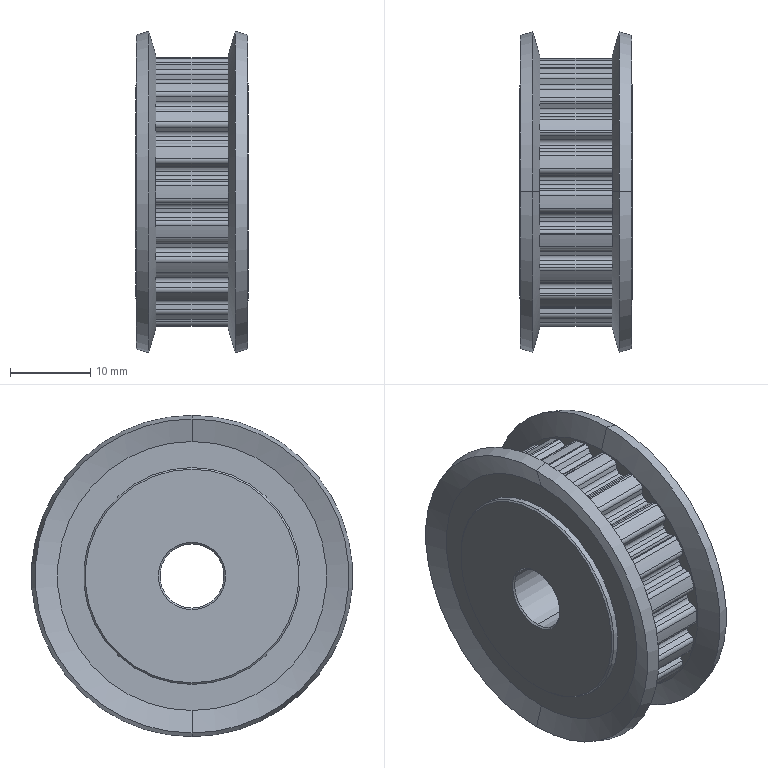Part | SolidWorks | features BaseBody 1 | 1 solid | 213 faces | box 14 x 40 x 40 mm | volume 11703 mm3 | cylinder 149 | plane 48 | cone 16 | commonest cylinder face diameters 1.22 x101 30.65 x21 33.45 x21 27 x4 8 x2